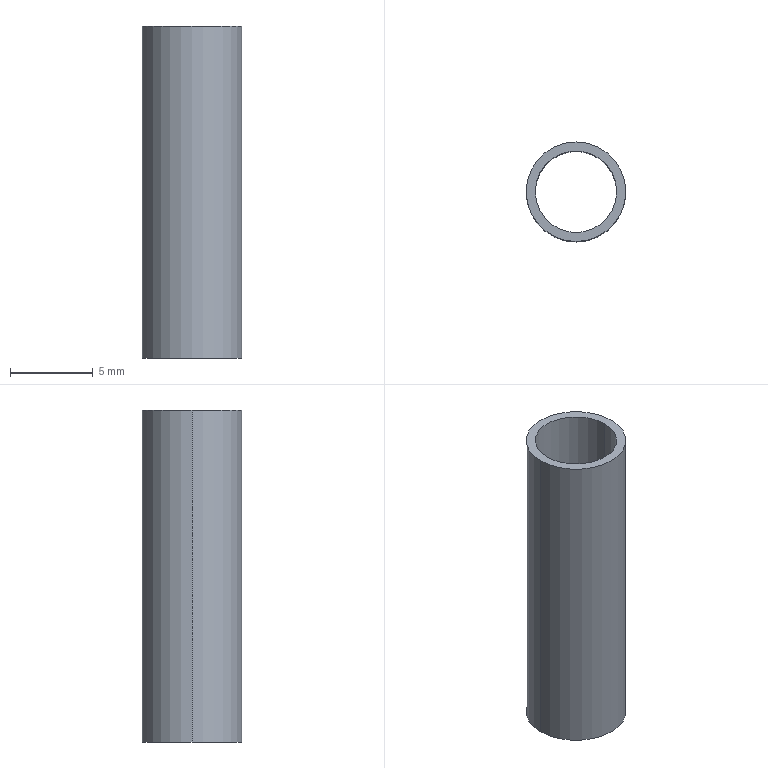Part | SolidWorks | features Extrusion 1 | 1 solid | 6 faces | box 6 x 6 x 20 mm | volume 188.338 mm3 | cylinder 4 | plane 2 | commonest cylinder face diameters 4.9 x2 6 x2
STEP:
#1=CARTESIAN_POINT('',(-2.45,0.,-20.));
#2=VERTEX_POINT('',#1);
#3=CARTESIAN_POINT('',(2.45,0.,-20.));
#4=VERTEX_POINT('',#3);
#5=CARTESIAN_POINT('',(0.,0.,-20.));
#6=DIRECTION('',(0.,0.,1.));
#7=DIRECTION('',(1.,0.,0.));
#8=AXIS2_PLACEMENT_3D('',#5,#6,#7);
#9=CIRCLE('',#8,2.45);
#10=EDGE_CURVE('',#2,#4,#9,.T.);
#11=ORIENTED_EDGE('',*,*,#10,.F.);
#12=CARTESIAN_POINT('',(-2.45,0.,0.));
#13=VERTEX_POINT('',#12);
#14=CARTESIAN_POINT('',(-2.45,0.,-28.485));
#15=DIRECTION('',(0.,0.,1.));
#16=VECTOR('',#15,1000.);
#17=LINE('',#14,#16);
#18=EDGE_CURVE('',#2,#13,#17,.T.);
#19=ORIENTED_EDGE('',*,*,#18,.T.);
#20=CARTESIAN_POINT('',(2.45,0.,0.));
#21=VERTEX_POINT('',#20);
#22=CARTESIAN_POINT('',(0.,0.,0.));
#23=DIRECTION('',(0.,0.,1.));
#24=DIRECTION('',(1.,0.,0.));
#25=AXIS2_PLACEMENT_3D('',#22,#23,#24);
#26=CIRCLE('',#25,2.45);
#27=EDGE_CURVE('',#13,#21,#26,.T.);
#28=ORIENTED_EDGE('',*,*,#27,.T.);
#29=CARTESIAN_POINT('',(2.45,0.,-28.485));
#30=DIRECTION('',(0.,0.,1.));
#31=VECTOR('',#30,1000.);
#32=LINE('',#29,#31);
#33=EDGE_CURVE('',#4,#21,#32,.T.);
#34=ORIENTED_EDGE('',*,*,#33,.F.);
#35=EDGE_LOOP('',(#11,#19,#28,#34));
#36=FACE_OUTER_BOUND('',#35,.T.);
#37=CARTESIAN_POINT('',(0.,0.,-28.485));
#38=DIRECTION('',(0.,0.,1.));
#39=DIRECTION('',(1.,0.,0.));
#40=AXIS2_PLACEMENT_3D('',#37,#38,#39);
#41=CYLINDRICAL_SURFACE('',#40,2.45);
#42=ADVANCED_FACE('',(#36),#41,.F.);
#43=CARTESIAN_POINT('',(-3.,0.,-20.));
#44=VERTEX_POINT('',#43);
#45=CARTESIAN_POINT('',(3.,0.,-20.));
#46=VERTEX_POINT('',#45);
#47=CARTESIAN_POINT('',(0.,0.,-20.));
#48=DIRECTION('',(0.,0.,-1.));
#49=DIRECTION('',(1.,0.,0.));
#50=AXIS2_PLACEMENT_3D('',#47,#48,#49);
#51=CIRCLE('',#50,3.);
#52=EDGE_CURVE('',#44,#46,#51,.T.);
#53=ORIENTED_EDGE('',*,*,#52,.F.);
#54=CARTESIAN_POINT('',(-3.,0.,0.));
#55=VERTEX_POINT('',#54);
#56=CARTESIAN_POINT('',(-3.,0.,-28.485));
#57=DIRECTION('',(0.,0.,1.));
#58=VECTOR('',#57,1000.);
#59=LINE('',#56,#58);
#60=EDGE_CURVE('',#44,#55,#59,.T.);
#61=ORIENTED_EDGE('',*,*,#60,.T.);
#62=CARTESIAN_POINT('',(3.,0.,0.));
#63=VERTEX_POINT('',#62);
#64=CARTESIAN_POINT('',(0.,0.,0.));
#65=DIRECTION('',(0.,0.,1.));
#66=DIRECTION('',(1.,0.,0.));
#67=AXIS2_PLACEMENT_3D('',#64,#65,#66);
#68=CIRCLE('',#67,3.);
#69=EDGE_CURVE('',#63,#55,#68,.T.);
#70=ORIENTED_EDGE('',*,*,#69,.F.);
#71=CARTESIAN_POINT('',(3.,0.,-28.485));
#72=DIRECTION('',(0.,0.,1.));
#73=VECTOR('',#72,1000.);
#74=LINE('',#71,#73);
#75=EDGE_CURVE('',#46,#63,#74,.T.);
#76=ORIENTED_EDGE('',*,*,#75,.F.);
#77=EDGE_LOOP('',(#53,#61,#70,#76));
#78=FACE_OUTER_BOUND('',#77,.T.);
#79=CARTESIAN_POINT('',(0.,0.,-28.485));
#80=DIRECTION('',(0.,0.,1.));
#81=DIRECTION('',(1.,0.,0.));
#82=AXIS2_PLACEMENT_3D('',#79,#80,#81);
#83=CYLINDRICAL_SURFACE('',#82,3.);
#84=ADVANCED_FACE('',(#78),#83,.T.);
#85=CARTESIAN_POINT('',(0.,0.,-20.));
#86=DIRECTION('',(0.,0.,-1.));
#87=DIRECTION('',(1.,0.,0.));
#88=AXIS2_PLACEMENT_3D('',#85,#86,#87);
#89=CIRCLE('',#88,3.);
#90=EDGE_CURVE('',#46,#44,#89,.T.);
#91=ORIENTED_EDGE('',*,*,#90,.T.);
#92=ORIENTED_EDGE('',*,*,#52,.T.);
#93=EDGE_LOOP('',(#91,#92));
#94=FACE_OUTER_BOUND('',#93,.T.);
#95=CARTESIAN_POINT('',(0.,0.,-20.));
#96=DIRECTION('',(0.,0.,1.));
#97=DIRECTION('',(1.,0.,0.));
#98=AXIS2_PLACEMENT_3D('',#95,#96,#97);
#99=CIRCLE('',#98,2.45);
#100=EDGE_CURVE('',#4,#2,#99,.T.);
#101=ORIENTED_EDGE('',*,*,#100,.T.);
#102=ORIENTED_EDGE('',*,*,#10,.T.);
#103=EDGE_LOOP('',(#101,#102));
#104=FACE_BOUND('',#103,.T.);
#105=CARTESIAN_POINT('',(0.,0.,-20.));
#106=DIRECTION('',(0.,0.,1.));
#107=DIRECTION('',(1.,0.,0.));
#108=AXIS2_PLACEMENT_3D('',#105,#106,#107);
#109=PLANE('',#108);
#110=ADVANCED_FACE('',(#94,#104),#109,.F.);
#111=ORIENTED_EDGE('',*,*,#60,.F.);
#112=ORIENTED_EDGE('',*,*,#90,.F.);
#113=ORIENTED_EDGE('',*,*,#75,.T.);
#114=CARTESIAN_POINT('',(0.,0.,0.));
#115=DIRECTION('',(0.,0.,1.));
#116=DIRECTION('',(1.,0.,0.));
#117=AXIS2_PLACEMENT_3D('',#114,#115,#116);
#118=CIRCLE('',#117,3.);
#119=EDGE_CURVE('',#55,#63,#118,.T.);
#120=ORIENTED_EDGE('',*,*,#119,.F.);
#121=EDGE_LOOP('',(#111,#112,#113,#120));
#122=FACE_OUTER_BOUND('',#121,.T.);
#123=CARTESIAN_POINT('',(0.,0.,-28.485));
#124=DIRECTION('',(0.,0.,1.));
#125=DIRECTION('',(1.,0.,0.));
#126=AXIS2_PLACEMENT_3D('',#123,#124,#125);
#127=CYLINDRICAL_SURFACE('',#126,3.);
#128=ADVANCED_FACE('',(#122),#127,.T.);
#129=CARTESIAN_POINT('',(0.,0.,0.));
#130=DIRECTION('',(0.,0.,1.));
#131=DIRECTION('',(1.,0.,0.));
#132=AXIS2_PLACEMENT_3D('',#129,#130,#131);
#133=CIRCLE('',#132,2.45);
#134=EDGE_CURVE('',#21,#13,#133,.T.);
#135=ORIENTED_EDGE('',*,*,#134,.F.);
#136=ORIENTED_EDGE('',*,*,#27,.F.);
#137=EDGE_LOOP('',(#135,#136));
#138=FACE_BOUND('',#137,.T.);
#139=ORIENTED_EDGE('',*,*,#69,.T.);
#140=ORIENTED_EDGE('',*,*,#119,.T.);
#141=EDGE_LOOP('',(#139,#140));
#142=FACE_OUTER_BOUND('',#141,.T.);
#143=CARTESIAN_POINT('',(0.,0.,0.));
#144=DIRECTION('',(0.,0.,1.));
#145=DIRECTION('',(1.,0.,0.));
#146=AXIS2_PLACEMENT_3D('',#143,#144,#145);
#147=PLANE('',#146);
#148=ADVANCED_FACE('',(#138,#142),#147,.T.);
#149=ORIENTED_EDGE('',*,*,#18,.F.);
#150=ORIENTED_EDGE('',*,*,#100,.F.);
#151=ORIENTED_EDGE('',*,*,#33,.T.);
#152=ORIENTED_EDGE('',*,*,#134,.T.);
#153=EDGE_LOOP('',(#149,#150,#151,#152));
#154=FACE_OUTER_BOUND('',#153,.T.);
#155=CARTESIAN_POINT('',(0.,0.,-28.485));
#156=DIRECTION('',(0.,0.,1.));
#157=DIRECTION('',(1.,0.,0.));
#158=AXIS2_PLACEMENT_3D('',#155,#156,#157);
#159=CYLINDRICAL_SURFACE('',#158,2.45);
#160=ADVANCED_FACE('',(#154),#159,.F.);
#161=CLOSED_SHELL('',(#42,#84,#110,#128,#148,#160));
#162=MANIFOLD_SOLID_BREP('',#161);
#163=CARTESIAN_POINT('',(0.,0.,0.));
#164=DIRECTION('',(0.,0.,1.));
#165=DIRECTION('',(1.,0.,0.));
#166=AXIS2_PLACEMENT_3D('',#163,#164,#165);
#167=(LENGTH_UNIT()NAMED_UNIT(*)SI_UNIT(.MILLI.,.METRE.));
#168=UNCERTAINTY_MEASURE_WITH_UNIT(LENGTH_MEASURE(0.00001),#167,'','');
#169=(NAMED_UNIT(*)PLANE_ANGLE_UNIT()SI_UNIT($,.RADIAN.));
#170=(NAMED_UNIT(*)SI_UNIT($,.STERADIAN.)SOLID_ANGLE_UNIT());
#171=(GEOMETRIC_REPRESENTATION_CONTEXT(3)GLOBAL_UNCERTAINTY_ASSIGNED_CONTEXT((#168))GLOBAL_UNIT_ASSIGNED_CONTEXT((#167,#169,#170))REPRESENTATION_CONTEXT('',''));
#172=ADVANCED_BREP_SHAPE_REPRESENTATION('',(#162,#166),#171);